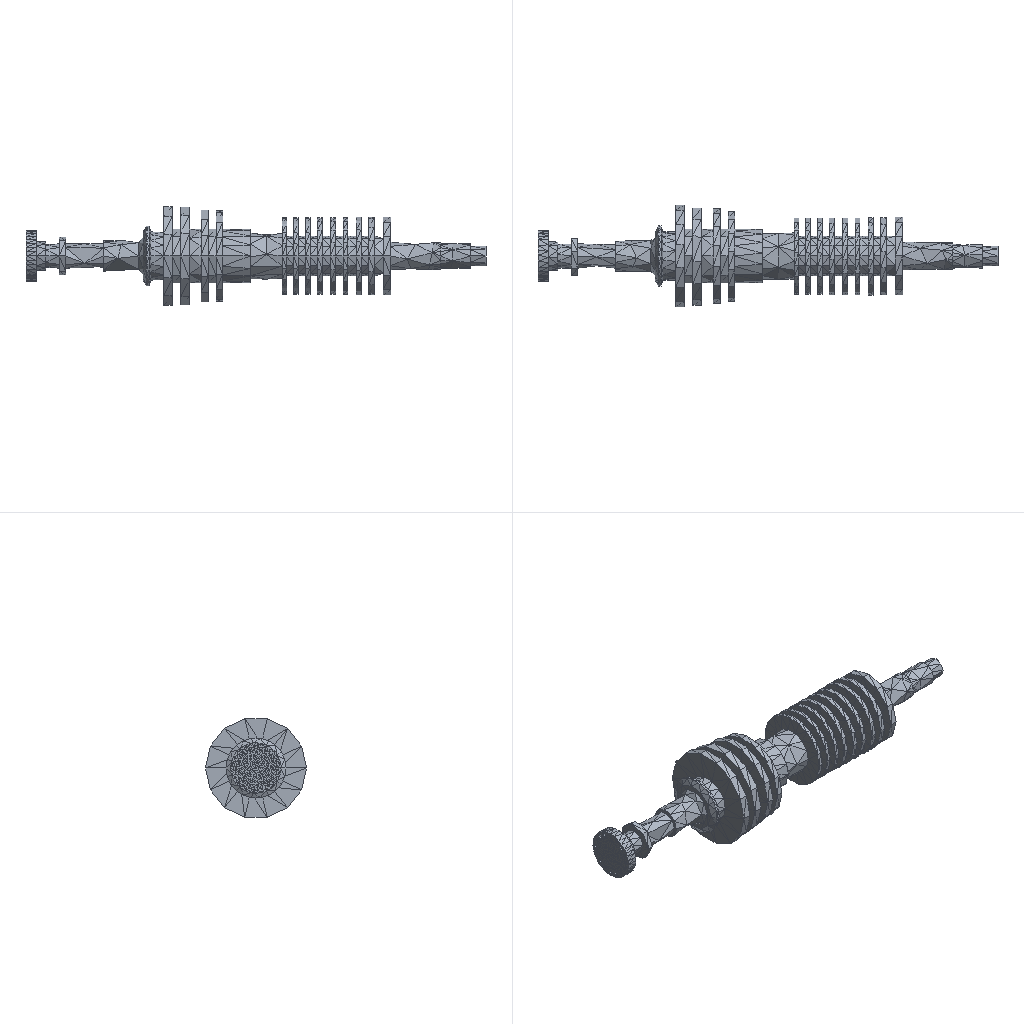Simulation study | ansys workbench
Set-up summary:
category,name,step,type,value,unit,region
solver,ansys_workbench
units,mm-N-s-tonne (MPa),,stated,"/units,MPA"
analysis,deck-1/LS1,,modal,method=damp; n_modes=12
load_step,deck-1/LS1,deck-1/LS1,modal
analysis,deck-2/LS1,,transient
load_step,deck-2/LS1,deck-2/LS1,transient,time=20
mesh,deck-1.dat,,nodes,17555
mesh,deck-1.dat,,elements,9763
element_type,SOLID187,,,9763,,deck-1.dat
mesh,deck-2.dat,,nodes,17556
mesh,deck-2.dat,,elements,9917
element_type,SOLID187,,,9763,,deck-2.dat
element_type,CONTA174,,,154,,deck-2.dat
material,Structural Steel,,E,200000,tonne s^-2 mm^-1
material,Structural Steel,,nu,0.3
material,Structural Steel,,density,7.85e-09,tonne mm^-3
material,Structural Steel,,conductivity,60.5,tonne mm s^-3 C^-1
material,Structural Steel,,specific_heat,4.34e+08,mm^2 s^-2 C^-1
material,Structural Steel,,cte,1.2e-05,C^-1
material,Structural Steel,,permeability,10000
material,Structural Steel,,resistivity,0.00017,ohm mm
material,Structural Steel,,E,200000,tonne s^-2 mm^-1
material,Structural Steel,,nu,0.3
material,Structural Steel,,density,7.85e-09,tonne mm^-3
material,Structural Steel,,conductivity,60.5,tonne mm s^-3 C^-1
material,Structural Steel,,specific_heat,4.34e+08,mm^2 s^-2 C^-1
material,Structural Steel,,cte,1.2e-05,C^-1
material,Structural Steel,,permeability,10000
material,Structural Steel,,resistivity,0.00017,ohm mm
load,,deck-2/LS1,moment,"150 [dir=(1, 0, 0) n=3]",,all
bc,Fixed Supports,deck-2/model,fixed,[dofs=ALL],,_FIXEDSU
contact,contact 1,,bonded (always),element=CONTA174
named_set,_FIXEDSU,,node,114
Results summary:
result,analyses[0].index,,,1
result,analyses[0].system,,,SYS
result,analyses[0].deck,,,deck-1.dat
result,analyses[0].solve_status,,,completed
result,analyses[0].analysis_type,,,modal
result,analyses[0].physics,,,mechanical
result,analyses[0].unit_system,,,"NMM: mm, ton, N, s, mV, mA, degC"
result,analyses[0].n_sets,,,12
result,analyses[0].modal_frequencies_hz[1],,,0
result,analyses[0].modal_frequencies_hz[2],,,0
result,analyses[0].modal_frequencies_hz[3],,,0
result,analyses[0].modal_frequencies_hz[4],,,0
result,analyses[0].modal_frequencies_hz[5],,,9.24102e-05
result,analyses[0].modal_frequencies_hz[6],,,-9.24102e-05
result,analyses[0].modal_frequencies_hz[7],,,0
result,analyses[0].modal_frequencies_hz[8],,,0
result,analyses[0].modal_frequencies_hz[9],,,0
result,analyses[0].modal_frequencies_hz[10],,,0
result,analyses[0].modal_frequencies_hz[11],,,0.0002816
result,analyses[0].modal_frequencies_hz[12],,,-0.0002816
result,analyses[1].index,,,2
result,analyses[1].system,,,SYS-1
result,analyses[1].deck,,,deck-2.dat
result,analyses[1].solve_status,,,completed
result,analyses[1].analysis_type,,,static
result,analyses[1].physics,,,mechanical
result,analyses[1].unit_system,,,"NMM: mm, ton, N, s, mV, mA, degC"
result,analyses[1].n_sets,,,1
result,analyses[1].load_steps[0].set,set=1,,1
result,analyses[1].load_steps[0].time_or_freq,set=1,,20
result,analyses[1].load_steps[0].max_displacement_magnitude,set=1,,5.77506e-08
result,analyses[1].load_steps[0].max_von_mises_nodal,set=1,,2.35757e-06
result,analyses[1].load_steps[0].reaction_force_sum_xyz[1],set=1,,1.76797e-10
result,analyses[1].load_steps[0].reaction_force_sum_xyz[2],set=1,,1.99398e-10
result,analyses[1].load_steps[0].reaction_force_sum_xyz[3],set=1,,-6.61242e-11
result,geometry_export[0][0],,,.step
result,geometry_export[0][1],,,ok
result,geometry_export[0][2],,,1